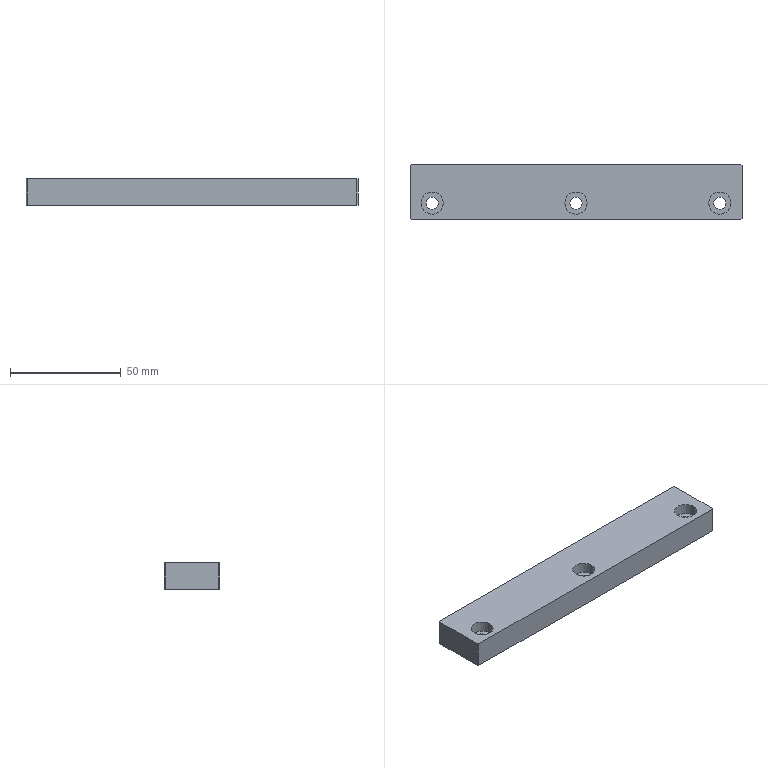Part | SolidWorks | features Chamfer 1, Extrusion 1, HoleWzd 1 | 1 solid | 25 faces | box 150 x 25 x 12 mm | volume 43317 mm3 | plane 13 | cylinder 12 | commonest cylinder face diameters 5.5 x6 10 x6
STEP:
#1=CARTESIAN_POINT('',(-5.,-5.,7.));
#2=VERTEX_POINT('',#1);
#3=CARTESIAN_POINT('',(5.,-5.,7.));
#4=VERTEX_POINT('',#3);
#5=CARTESIAN_POINT('',(0.,-5.,7.));
#6=DIRECTION('',(0.,0.,1.));
#7=DIRECTION('',(1.,0.,0.));
#8=AXIS2_PLACEMENT_3D('',#5,#6,#7);
#9=CIRCLE('',#8,5.);
#10=EDGE_CURVE('',#2,#4,#9,.T.);
#11=ORIENTED_EDGE('',*,*,#10,.F.);
#12=CARTESIAN_POINT('',(-5.,-5.,12.));
#13=VERTEX_POINT('',#12);
#14=CARTESIAN_POINT('',(-5.,-5.,12.));
#15=DIRECTION('',(0.,0.,1.));
#16=VECTOR('',#15,1000.);
#17=LINE('',#14,#16);
#18=EDGE_CURVE('',#2,#13,#17,.T.);
#19=ORIENTED_EDGE('',*,*,#18,.T.);
#20=CARTESIAN_POINT('',(5.,-5.,12.));
#21=VERTEX_POINT('',#20);
#22=CARTESIAN_POINT('',(0.,-5.,12.));
#23=DIRECTION('',(0.,0.,1.));
#24=DIRECTION('',(1.,0.,0.));
#25=AXIS2_PLACEMENT_3D('',#22,#23,#24);
#26=CIRCLE('',#25,5.);
#27=EDGE_CURVE('',#13,#21,#26,.T.);
#28=ORIENTED_EDGE('',*,*,#27,.T.);
#29=CARTESIAN_POINT('',(5.,-5.,12.));
#30=DIRECTION('',(0.,0.,1.));
#31=VECTOR('',#30,1000.);
#32=LINE('',#29,#31);
#33=EDGE_CURVE('',#4,#21,#32,.T.);
#34=ORIENTED_EDGE('',*,*,#33,.F.);
#35=EDGE_LOOP('',(#11,#19,#28,#34));
#36=FACE_OUTER_BOUND('',#35,.T.);
#37=CARTESIAN_POINT('',(0.,-5.,12.));
#38=DIRECTION('',(0.,0.,1.));
#39=DIRECTION('',(1.,0.,0.));
#40=AXIS2_PLACEMENT_3D('',#37,#38,#39);
#41=CYLINDRICAL_SURFACE('',#40,5.);
#42=ADVANCED_FACE('',(#36),#41,.F.);
#43=CARTESIAN_POINT('',(-2.75,-5.,0.));
#44=VERTEX_POINT('',#43);
#45=CARTESIAN_POINT('',(2.75,-5.,0.));
#46=VERTEX_POINT('',#45);
#47=CARTESIAN_POINT('',(0.,-5.,0.));
#48=DIRECTION('',(0.,0.,1.));
#49=DIRECTION('',(1.,0.,0.));
#50=AXIS2_PLACEMENT_3D('',#47,#48,#49);
#51=CIRCLE('',#50,2.75);
#52=EDGE_CURVE('',#44,#46,#51,.T.);
#53=ORIENTED_EDGE('',*,*,#52,.F.);
#54=CARTESIAN_POINT('',(-2.75,-5.,7.));
#55=VERTEX_POINT('',#54);
#56=CARTESIAN_POINT('',(-2.75,-5.,12.));
#57=DIRECTION('',(0.,0.,1.));
#58=VECTOR('',#57,1000.);
#59=LINE('',#56,#58);
#60=EDGE_CURVE('',#44,#55,#59,.T.);
#61=ORIENTED_EDGE('',*,*,#60,.T.);
#62=CARTESIAN_POINT('',(2.75,-5.,7.));
#63=VERTEX_POINT('',#62);
#64=CARTESIAN_POINT('',(0.,-5.,7.));
#65=DIRECTION('',(0.,0.,1.));
#66=DIRECTION('',(1.,0.,0.));
#67=AXIS2_PLACEMENT_3D('',#64,#65,#66);
#68=CIRCLE('',#67,2.75);
#69=EDGE_CURVE('',#55,#63,#68,.T.);
#70=ORIENTED_EDGE('',*,*,#69,.T.);
#71=CARTESIAN_POINT('',(2.75,-5.,12.));
#72=DIRECTION('',(0.,0.,1.));
#73=VECTOR('',#72,1000.);
#74=LINE('',#71,#73);
#75=EDGE_CURVE('',#46,#63,#74,.T.);
#76=ORIENTED_EDGE('',*,*,#75,.F.);
#77=EDGE_LOOP('',(#53,#61,#70,#76));
#78=FACE_OUTER_BOUND('',#77,.T.);
#79=CARTESIAN_POINT('',(0.,-5.,12.));
#80=DIRECTION('',(0.,0.,1.));
#81=DIRECTION('',(1.,0.,0.));
#82=AXIS2_PLACEMENT_3D('',#79,#80,#81);
#83=CYLINDRICAL_SURFACE('',#82,2.75);
#84=ADVANCED_FACE('',(#78),#83,.F.);
#85=CARTESIAN_POINT('',(-70.,-5.,7.));
#86=VERTEX_POINT('',#85);
#87=CARTESIAN_POINT('',(-60.,-5.,7.));
#88=VERTEX_POINT('',#87);
#89=CARTESIAN_POINT('',(-65.,-5.,7.));
#90=DIRECTION('',(0.,0.,1.));
#91=DIRECTION('',(1.,0.,0.));
#92=AXIS2_PLACEMENT_3D('',#89,#90,#91);
#93=CIRCLE('',#92,5.);
#94=EDGE_CURVE('',#86,#88,#93,.T.);
#95=ORIENTED_EDGE('',*,*,#94,.F.);
#96=CARTESIAN_POINT('',(-70.,-5.,12.));
#97=VERTEX_POINT('',#96);
#98=CARTESIAN_POINT('',(-70.,-5.,12.));
#99=DIRECTION('',(0.,0.,1.));
#100=VECTOR('',#99,1000.);
#101=LINE('',#98,#100);
#102=EDGE_CURVE('',#86,#97,#101,.T.);
#103=ORIENTED_EDGE('',*,*,#102,.T.);
#104=CARTESIAN_POINT('',(-60.,-5.,12.));
#105=VERTEX_POINT('',#104);
#106=CARTESIAN_POINT('',(-65.,-5.,12.));
#107=DIRECTION('',(0.,0.,1.));
#108=DIRECTION('',(1.,0.,0.));
#109=AXIS2_PLACEMENT_3D('',#106,#107,#108);
#110=CIRCLE('',#109,5.);
#111=EDGE_CURVE('',#97,#105,#110,.T.);
#112=ORIENTED_EDGE('',*,*,#111,.T.);
#113=CARTESIAN_POINT('',(-60.,-5.,12.));
#114=DIRECTION('',(0.,0.,1.));
#115=VECTOR('',#114,1000.);
#116=LINE('',#113,#115);
#117=EDGE_CURVE('',#88,#105,#116,.T.);
#118=ORIENTED_EDGE('',*,*,#117,.F.);
#119=EDGE_LOOP('',(#95,#103,#112,#118));
#120=FACE_OUTER_BOUND('',#119,.T.);
#121=CARTESIAN_POINT('',(-65.,-5.,12.));
#122=DIRECTION('',(0.,0.,1.));
#123=DIRECTION('',(1.,0.,0.));
#124=AXIS2_PLACEMENT_3D('',#121,#122,#123);
#125=CYLINDRICAL_SURFACE('',#124,5.);
#126=ADVANCED_FACE('',(#120),#125,.F.);
#127=CARTESIAN_POINT('',(-67.75,-5.,0.));
#128=VERTEX_POINT('',#127);
#129=CARTESIAN_POINT('',(-62.25,-5.,0.));
#130=VERTEX_POINT('',#129);
#131=CARTESIAN_POINT('',(-65.,-5.,0.));
#132=DIRECTION('',(0.,0.,1.));
#133=DIRECTION('',(1.,0.,0.));
#134=AXIS2_PLACEMENT_3D('',#131,#132,#133);
#135=CIRCLE('',#134,2.75);
#136=EDGE_CURVE('',#128,#130,#135,.T.);
#137=ORIENTED_EDGE('',*,*,#136,.F.);
#138=CARTESIAN_POINT('',(-67.75,-5.,7.));
#139=VERTEX_POINT('',#138);
#140=CARTESIAN_POINT('',(-67.75,-5.,12.));
#141=DIRECTION('',(0.,0.,1.));
#142=VECTOR('',#141,1000.);
#143=LINE('',#140,#142);
#144=EDGE_CURVE('',#128,#139,#143,.T.);
#145=ORIENTED_EDGE('',*,*,#144,.T.);
#146=CARTESIAN_POINT('',(-62.25,-5.,7.));
#147=VERTEX_POINT('',#146);
#148=CARTESIAN_POINT('',(-65.,-5.,7.));
#149=DIRECTION('',(0.,0.,1.));
#150=DIRECTION('',(1.,0.,0.));
#151=AXIS2_PLACEMENT_3D('',#148,#149,#150);
#152=CIRCLE('',#151,2.75);
#153=EDGE_CURVE('',#139,#147,#152,.T.);
#154=ORIENTED_EDGE('',*,*,#153,.T.);
#155=CARTESIAN_POINT('',(-62.25,-5.,12.));
#156=DIRECTION('',(0.,0.,1.));
#157=VECTOR('',#156,1000.);
#158=LINE('',#155,#157);
#159=EDGE_CURVE('',#130,#147,#158,.T.);
#160=ORIENTED_EDGE('',*,*,#159,.F.);
#161=EDGE_LOOP('',(#137,#145,#154,#160));
#162=FACE_OUTER_BOUND('',#161,.T.);
#163=CARTESIAN_POINT('',(-65.,-5.,12.));
#164=DIRECTION('',(0.,0.,1.));
#165=DIRECTION('',(1.,0.,0.));
#166=AXIS2_PLACEMENT_3D('',#163,#164,#165);
#167=CYLINDRICAL_SURFACE('',#166,2.75);
#168=ADVANCED_FACE('',(#162),#167,.F.);
#169=CARTESIAN_POINT('',(60.,-5.,7.));
#170=VERTEX_POINT('',#169);
#171=CARTESIAN_POINT('',(70.,-5.,7.));
#172=VERTEX_POINT('',#171);
#173=CARTESIAN_POINT('',(65.,-5.,7.));
#174=DIRECTION('',(0.,0.,1.));
#175=DIRECTION('',(1.,0.,0.));
#176=AXIS2_PLACEMENT_3D('',#173,#174,#175);
#177=CIRCLE('',#176,5.);
#178=EDGE_CURVE('',#170,#172,#177,.T.);
#179=ORIENTED_EDGE('',*,*,#178,.F.);
#180=CARTESIAN_POINT('',(60.,-5.,12.));
#181=VERTEX_POINT('',#180);
#182=CARTESIAN_POINT('',(60.,-5.,12.));
#183=DIRECTION('',(0.,0.,1.));
#184=VECTOR('',#183,1000.);
#185=LINE('',#182,#184);
#186=EDGE_CURVE('',#170,#181,#185,.T.);
#187=ORIENTED_EDGE('',*,*,#186,.T.);
#188=CARTESIAN_POINT('',(70.,-5.,12.));
#189=VERTEX_POINT('',#188);
#190=CARTESIAN_POINT('',(65.,-5.,12.));
#191=DIRECTION('',(0.,0.,1.));
#192=DIRECTION('',(1.,0.,0.));
#193=AXIS2_PLACEMENT_3D('',#190,#191,#192);
#194=CIRCLE('',#193,5.);
#195=EDGE_CURVE('',#181,#189,#194,.T.);
#196=ORIENTED_EDGE('',*,*,#195,.T.);
#197=CARTESIAN_POINT('',(70.,-5.,12.));
#198=DIRECTION('',(0.,0.,1.));
#199=VECTOR('',#198,1000.);
#200=LINE('',#197,#199);
#201=EDGE_CURVE('',#172,#189,#200,.T.);
#202=ORIENTED_EDGE('',*,*,#201,.F.);
#203=EDGE_LOOP('',(#179,#187,#196,#202));
#204=FACE_OUTER_BOUND('',#203,.T.);
#205=CARTESIAN_POINT('',(65.,-5.,12.));
#206=DIRECTION('',(0.,0.,1.));
#207=DIRECTION('',(1.,0.,0.));
#208=AXIS2_PLACEMENT_3D('',#205,#206,#207);
#209=CYLINDRICAL_SURFACE('',#208,5.);
#210=ADVANCED_FACE('',(#204),#209,.F.);
#211=CARTESIAN_POINT('',(62.25,-5.,0.));
#212=VERTEX_POINT('',#211);
#213=CARTESIAN_POINT('',(67.75,-5.,0.));
#214=VERTEX_POINT('',#213);
#215=CARTESIAN_POINT('',(65.,-5.,0.));
#216=DIRECTION('',(0.,0.,1.));
#217=DIRECTION('',(1.,0.,0.));
#218=AXIS2_PLACEMENT_3D('',#215,#216,#217);
#219=CIRCLE('',#218,2.75);
#220=EDGE_CURVE('',#212,#214,#219,.T.);
#221=ORIENTED_EDGE('',*,*,#220,.F.);
#222=CARTESIAN_POINT('',(62.25,-5.,7.));
#223=VERTEX_POINT('',#222);
#224=CARTESIAN_POINT('',(62.25,-5.,12.));
#225=DIRECTION('',(0.,0.,1.));
#226=VECTOR('',#225,1000.);
#227=LINE('',#224,#226);
#228=EDGE_CURVE('',#212,#223,#227,.T.);
#229=ORIENTED_EDGE('',*,*,#228,.T.);
#230=CARTESIAN_POINT('',(67.75,-5.,7.));
#231=VERTEX_POINT('',#230);
#232=CARTESIAN_POINT('',(65.,-5.,7.));
#233=DIRECTION('',(0.,0.,1.));
#234=DIRECTION('',(1.,0.,0.));
#235=AXIS2_PLACEMENT_3D('',#232,#233,#234);
#236=CIRCLE('',#235,2.75);
#237=EDGE_CURVE('',#223,#231,#236,.T.);
#238=ORIENTED_EDGE('',*,*,#237,.T.);
#239=CARTESIAN_POINT('',(67.75,-5.,12.));
#240=DIRECTION('',(0.,0.,1.));
#241=VECTOR('',#240,1000.);
#242=LINE('',#239,#241);
#243=EDGE_CURVE('',#214,#231,#242,.T.);
#244=ORIENTED_EDGE('',*,*,#243,.F.);
#245=EDGE_LOOP('',(#221,#229,#238,#244));
#246=FACE_OUTER_BOUND('',#245,.T.);
#247=CARTESIAN_POINT('',(65.,-5.,12.));
#248=DIRECTION('',(0.,0.,1.));
#249=DIRECTION('',(1.,0.,0.));
#250=AXIS2_PLACEMENT_3D('',#247,#248,#249);
#251=CYLINDRICAL_SURFACE('',#250,2.75);
#252=ADVANCED_FACE('',(#246),#251,.F.);
#253=CARTESIAN_POINT('',(75.,-12.,12.));
#254=VERTEX_POINT('',#253);
#255=CARTESIAN_POINT('',(75.,12.,12.));
#256=VERTEX_POINT('',#255);
#257=CARTESIAN_POINT('',(75.,12.5,12.));
#258=DIRECTION('',(0.,1.,0.));
#259=VECTOR('',#258,1000.);
#260=LINE('',#257,#259);
#261=EDGE_CURVE('',#254,#256,#260,.T.);
#262=ORIENTED_EDGE('',*,*,#261,.F.);
#263=CARTESIAN_POINT('',(75.,-12.,0.));
#264=VERTEX_POINT('',#263);
#265=CARTESIAN_POINT('',(75.,-12.,12.));
#266=DIRECTION('',(0.,0.,-1.));
#267=VECTOR('',#266,1000.);
#268=LINE('',#265,#267);
#269=EDGE_CURVE('',#254,#264,#268,.T.);
#270=ORIENTED_EDGE('',*,*,#269,.T.);
#271=CARTESIAN_POINT('',(75.,12.,0.));
#272=VERTEX_POINT('',#271);
#273=CARTESIAN_POINT('',(75.,12.5,0.));
#274=DIRECTION('',(0.,1.,0.));
#275=VECTOR('',#274,1000.);
#276=LINE('',#273,#275);
#277=EDGE_CURVE('',#264,#272,#276,.T.);
#278=ORIENTED_EDGE('',*,*,#277,.T.);
#279=CARTESIAN_POINT('',(75.,12.,12.));
#280=DIRECTION('',(0.,0.,1.));
#281=VECTOR('',#280,1000.);
#282=LINE('',#279,#281);
#283=EDGE_CURVE('',#272,#256,#282,.T.);
#284=ORIENTED_EDGE('',*,*,#283,.T.);
#285=EDGE_LOOP('',(#262,#270,#278,#284));
#286=FACE_OUTER_BOUND('',#285,.T.);
#287=CARTESIAN_POINT('',(75.,12.5,12.));
#288=DIRECTION('',(-1.,0.,0.));
#289=DIRECTION('',(0.,0.,1.));
#290=AXIS2_PLACEMENT_3D('',#287,#288,#289);
#291=PLANE('',#290);
#292=ADVANCED_FACE('',(#286),#291,.F.);
#293=CARTESIAN_POINT('',(74.5,12.5,12.));
#294=VERTEX_POINT('',#293);
#295=CARTESIAN_POINT('',(-74.5,12.5,12.));
#296=VERTEX_POINT('',#295);
#297=CARTESIAN_POINT('',(-75.,12.5,12.));
#298=DIRECTION('',(-1.,0.,0.));
#299=VECTOR('',#298,1000.);
#300=LINE('',#297,#299);
#301=EDGE_CURVE('',#294,#296,#300,.T.);
#302=ORIENTED_EDGE('',*,*,#301,.F.);
#303=CARTESIAN_POINT('',(74.5,12.5,0.));
#304=VERTEX_POINT('',#303);
#305=CARTESIAN_POINT('',(74.5,12.5,12.));
#306=DIRECTION('',(0.,0.,-1.));
#307=VECTOR('',#306,1000.);
#308=LINE('',#305,#307);
#309=EDGE_CURVE('',#294,#304,#308,.T.);
#310=ORIENTED_EDGE('',*,*,#309,.T.);
#311=CARTESIAN_POINT('',(-74.5,12.5,0.));
#312=VERTEX_POINT('',#311);
#313=CARTESIAN_POINT('',(-75.,12.5,0.));
#314=DIRECTION('',(-1.,0.,0.));
#315=VECTOR('',#314,1000.);
#316=LINE('',#313,#315);
#317=EDGE_CURVE('',#304,#312,#316,.T.);
#318=ORIENTED_EDGE('',*,*,#317,.T.);
#319=CARTESIAN_POINT('',(-74.5,12.5,12.));
#320=DIRECTION('',(0.,0.,1.));
#321=VECTOR('',#320,1000.);
#322=LINE('',#319,#321);
#323=EDGE_CURVE('',#312,#296,#322,.T.);
#324=ORIENTED_EDGE('',*,*,#323,.T.);
#325=EDGE_LOOP('',(#302,#310,#318,#324));
#326=FACE_OUTER_BOUND('',#325,.T.);
#327=CARTESIAN_POINT('',(-75.,12.5,12.));
#328=DIRECTION('',(0.,-1.,0.));
#329=DIRECTION('',(0.,0.,-1.));
#330=AXIS2_PLACEMENT_3D('',#327,#328,#329);
#331=PLANE('',#330);
#332=ADVANCED_FACE('',(#326),#331,.F.);
#333=CARTESIAN_POINT('',(-75.,12.,12.));
#334=VERTEX_POINT('',#333);
#335=CARTESIAN_POINT('',(-75.,-12.,12.));
#336=VERTEX_POINT('',#335);
#337=CARTESIAN_POINT('',(-75.,12.5,12.));
#338=DIRECTION('',(0.,-1.,0.));
#339=VECTOR('',#338,1000.);
#340=LINE('',#337,#339);
#341=EDGE_CURVE('',#334,#336,#340,.T.);
#342=ORIENTED_EDGE('',*,*,#341,.F.);
#343=CARTESIAN_POINT('',(-75.,12.,0.));
#344=VERTEX_POINT('',#343);
#345=CARTESIAN_POINT('',(-75.,12.,12.));
#346=DIRECTION('',(0.,0.,-1.));
#347=VECTOR('',#346,1000.);
#348=LINE('',#345,#347);
#349=EDGE_CURVE('',#334,#344,#348,.T.);
#350=ORIENTED_EDGE('',*,*,#349,.T.);
#351=CARTESIAN_POINT('',(-75.,-12.,0.));
#352=VERTEX_POINT('',#351);
#353=CARTESIAN_POINT('',(-75.,12.5,0.));
#354=DIRECTION('',(0.,-1.,0.));
#355=VECTOR('',#354,1000.);
#356=LINE('',#353,#355);
#357=EDGE_CURVE('',#344,#352,#356,.T.);
#358=ORIENTED_EDGE('',*,*,#357,.T.);
#359=CARTESIAN_POINT('',(-75.,-12.,12.));
#360=DIRECTION('',(0.,0.,1.));
#361=VECTOR('',#360,1000.);
#362=LINE('',#359,#361);
#363=EDGE_CURVE('',#352,#336,#362,.T.);
#364=ORIENTED_EDGE('',*,*,#363,.T.);
#365=EDGE_LOOP('',(#342,#350,#358,#364));
#366=FACE_OUTER_BOUND('',#365,.T.);
#367=CARTESIAN_POINT('',(-75.,12.5,12.));
#368=DIRECTION('',(1.,0.,0.));
#369=DIRECTION('',(0.,0.,-1.));
#370=AXIS2_PLACEMENT_3D('',#367,#368,#369);
#371=PLANE('',#370);
#372=ADVANCED_FACE('',(#366),#371,.F.);
#373=CARTESIAN_POINT('',(-74.5,-12.5,0.));
#374=VERTEX_POINT('',#373);
#375=CARTESIAN_POINT('',(74.5,-12.5,0.));
#376=VERTEX_POINT('',#375);
#377=CARTESIAN_POINT('',(-75.,-12.5,0.));
#378=DIRECTION('',(1.,0.,0.));
#379=VECTOR('',#378,1000.);
#380=LINE('',#377,#379);
#381=EDGE_CURVE('',#374,#376,#380,.T.);
#382=ORIENTED_EDGE('',*,*,#381,.T.);
#383=CARTESIAN_POINT('',(74.5,-12.5,12.));
#384=VERTEX_POINT('',#383);
#385=CARTESIAN_POINT('',(74.5,-12.5,12.));
#386=DIRECTION('',(0.,0.,1.));
#387=VECTOR('',#386,1000.);
#388=LINE('',#385,#387);
#389=EDGE_CURVE('',#376,#384,#388,.T.);
#390=ORIENTED_EDGE('',*,*,#389,.T.);
#391=CARTESIAN_POINT('',(-74.5,-12.5,12.));
#392=VERTEX_POINT('',#391);
#393=CARTESIAN_POINT('',(-75.,-12.5,12.));
#394=DIRECTION('',(1.,0.,0.));
#395=VECTOR('',#394,1000.);
#396=LINE('',#393,#395);
#397=EDGE_CURVE('',#392,#384,#396,.T.);
#398=ORIENTED_EDGE('',*,*,#397,.F.);
#399=CARTESIAN_POINT('',(-74.5,-12.5,12.));
#400=DIRECTION('',(0.,0.,-1.));
#401=VECTOR('',#400,1000.);
#402=LINE('',#399,#401);
#403=EDGE_CURVE('',#392,#374,#402,.T.);
#404=ORIENTED_EDGE('',*,*,#403,.T.);
#405=EDGE_LOOP('',(#382,#390,#398,#404));
#406=FACE_OUTER_BOUND('',#405,.T.);
#407=CARTESIAN_POINT('',(-75.,-12.5,12.));
#408=DIRECTION('',(0.,1.,0.));
#409=DIRECTION('',(0.,0.,1.));
#410=AXIS2_PLACEMENT_3D('',#407,#408,#409);
#411=PLANE('',#410);
#412=ADVANCED_FACE('',(#406),#411,.F.);
#413=CARTESIAN_POINT('',(0.,-5.,12.));
#414=DIRECTION('',(0.,0.,1.));
#415=DIRECTION('',(1.,0.,0.));
#416=AXIS2_PLACEMENT_3D('',#413,#414,#415);
#417=CIRCLE('',#416,5.);
#418=EDGE_CURVE('',#21,#13,#417,.T.);
#419=ORIENTED_EDGE('',*,*,#418,.F.);
#420=ORIENTED_EDGE('',*,*,#27,.F.);
#421=EDGE_LOOP('',(#419,#420));
#422=FACE_BOUND('',#421,.T.);
#423=CARTESIAN_POINT('',(-65.,-5.,12.));
#424=DIRECTION('',(0.,0.,1.));
#425=DIRECTION('',(1.,0.,0.));
#426=AXIS2_PLACEMENT_3D('',#423,#424,#425);
#427=CIRCLE('',#426,5.);
#428=EDGE_CURVE('',#105,#97,#427,.T.);
#429=ORIENTED_EDGE('',*,*,#428,.F.);
#430=ORIENTED_EDGE('',*,*,#111,.F.);
#431=EDGE_LOOP('',(#429,#430));
#432=FACE_BOUND('',#431,.T.);
#433=CARTESIAN_POINT('',(65.,-5.,12.));
#434=DIRECTION('',(0.,0.,1.));
#435=DIRECTION('',(1.,0.,0.));
#436=AXIS2_PLACEMENT_3D('',#433,#434,#435);
#437=CIRCLE('',#436,5.);
#438=EDGE_CURVE('',#189,#181,#437,.T.);
#439=ORIENTED_EDGE('',*,*,#438,.F.);
#440=ORIENTED_EDGE('',*,*,#195,.F.);
#441=EDGE_LOOP('',(#439,#440));
#442=FACE_BOUND('',#441,.T.);
#443=ORIENTED_EDGE('',*,*,#397,.T.);
#444=CARTESIAN_POINT('',(74.75,-12.25,12.));
#445=DIRECTION('',(0.7071,0.7071,0.));
#446=VECTOR('',#445,1000.);
#447=LINE('',#444,#446);
#448=EDGE_CURVE('',#384,#254,#447,.T.);
#449=ORIENTED_EDGE('',*,*,#448,.T.);
#450=ORIENTED_EDGE('',*,*,#261,.T.);
#451=CARTESIAN_POINT('',(87.25,-0.25,12.));
#452=DIRECTION('',(-0.7071,0.7071,0.));
#453=VECTOR('',#452,1000.);
#454=LINE('',#451,#453);
#455=EDGE_CURVE('',#256,#294,#454,.T.);
#456=ORIENTED_EDGE('',*,*,#455,.T.);
#457=ORIENTED_EDGE('',*,*,#301,.T.);
#458=CARTESIAN_POINT('',(-12.25,74.75,12.));
#459=DIRECTION('',(-0.7071,-0.7071,0.));
#460=VECTOR('',#459,1000.);
#461=LINE('',#458,#460);
#462=EDGE_CURVE('',#296,#334,#461,.T.);
#463=ORIENTED_EDGE('',*,*,#462,.T.);
#464=ORIENTED_EDGE('',*,*,#341,.T.);
#465=CARTESIAN_POINT('',(0.25,-87.25,12.));
#466=DIRECTION('',(0.7071,-0.7071,0.));
#467=VECTOR('',#466,1000.);
#468=LINE('',#465,#467);
#469=EDGE_CURVE('',#336,#392,#468,.T.);
#470=ORIENTED_EDGE('',*,*,#469,.T.);
#471=EDGE_LOOP('',(#443,#449,#450,#456,#457,#463,#464,#470));
#472=FACE_OUTER_BOUND('',#471,.T.);
#473=CARTESIAN_POINT('',(75.,-12.5,12.));
#474=DIRECTION('',(0.,0.,1.));
#475=DIRECTION('',(1.,0.,0.));
#476=AXIS2_PLACEMENT_3D('',#473,#474,#475);
#477=PLANE('',#476);
#478=ADVANCED_FACE('',(#422,#432,#442,#472),#477,.T.);
#479=CARTESIAN_POINT('',(0.,-5.,0.));
#480=DIRECTION('',(0.,0.,1.));
#481=DIRECTION('',(1.,0.,0.));
#482=AXIS2_PLACEMENT_3D('',#479,#480,#481);
#483=CIRCLE('',#482,2.75);
#484=EDGE_CURVE('',#46,#44,#483,.T.);
#485=ORIENTED_EDGE('',*,*,#484,.T.);
#486=ORIENTED_EDGE('',*,*,#52,.T.);
#487=EDGE_LOOP('',(#485,#486));
#488=FACE_BOUND('',#487,.T.);
#489=CARTESIAN_POINT('',(-65.,-5.,0.));
#490=DIRECTION('',(0.,0.,1.));
#491=DIRECTION('',(1.,0.,0.));
#492=AXIS2_PLACEMENT_3D('',#489,#490,#491);
#493=CIRCLE('',#492,2.75);
#494=EDGE_CURVE('',#130,#128,#493,.T.);
#495=ORIENTED_EDGE('',*,*,#494,.T.);
#496=ORIENTED_EDGE('',*,*,#136,.T.);
#497=EDGE_LOOP('',(#495,#496));
#498=FACE_BOUND('',#497,.T.);
#499=CARTESIAN_POINT('',(65.,-5.,0.));
#500=DIRECTION('',(0.,0.,1.));
#501=DIRECTION('',(1.,0.,0.));
#502=AXIS2_PLACEMENT_3D('',#499,#500,#501);
#503=CIRCLE('',#502,2.75);
#504=EDGE_CURVE('',#214,#212,#503,.T.);
#505=ORIENTED_EDGE('',*,*,#504,.T.);
#506=ORIENTED_EDGE('',*,*,#220,.T.);
#507=EDGE_LOOP('',(#505,#506));
#508=FACE_BOUND('',#507,.T.);
#509=ORIENTED_EDGE('',*,*,#277,.F.);
#510=CARTESIAN_POINT('',(75.,-12.,0.));
#511=DIRECTION('',(-0.7071,-0.7071,0.));
#512=VECTOR('',#511,1000.);
#513=LINE('',#510,#512);
#514=EDGE_CURVE('',#264,#376,#513,.T.);
#515=ORIENTED_EDGE('',*,*,#514,.T.);
#516=ORIENTED_EDGE('',*,*,#381,.F.);
#517=CARTESIAN_POINT('',(-74.5,-12.5,0.));
#518=DIRECTION('',(-0.7071,0.7071,0.));
#519=VECTOR('',#518,1000.);
#520=LINE('',#517,#519);
#521=EDGE_CURVE('',#374,#352,#520,.T.);
#522=ORIENTED_EDGE('',*,*,#521,.T.);
#523=ORIENTED_EDGE('',*,*,#357,.F.);
#524=CARTESIAN_POINT('',(-75.,12.,0.));
#525=DIRECTION('',(0.7071,0.7071,0.));
#526=VECTOR('',#525,1000.);
#527=LINE('',#524,#526);
#528=EDGE_CURVE('',#344,#312,#527,.T.);
#529=ORIENTED_EDGE('',*,*,#528,.T.);
#530=ORIENTED_EDGE('',*,*,#317,.F.);
#531=CARTESIAN_POINT('',(74.5,12.5,0.));
#532=DIRECTION('',(0.7071,-0.7071,0.));
#533=VECTOR('',#532,1000.);
#534=LINE('',#531,#533);
#535=EDGE_CURVE('',#304,#272,#534,.T.);
#536=ORIENTED_EDGE('',*,*,#535,.T.);
#537=EDGE_LOOP('',(#509,#515,#516,#522,#523,#529,#530,#536));
#538=FACE_OUTER_BOUND('',#537,.T.);
#539=CARTESIAN_POINT('',(75.,-12.5,0.));
#540=DIRECTION('',(0.,0.,1.));
#541=DIRECTION('',(1.,0.,0.));
#542=AXIS2_PLACEMENT_3D('',#539,#540,#541);
#543=PLANE('',#542);
#544=ADVANCED_FACE('',(#488,#498,#508,#538),#543,.F.);
#545=ORIENTED_EDGE('',*,*,#228,.F.);
#546=ORIENTED_EDGE('',*,*,#504,.F.);
#547=ORIENTED_EDGE('',*,*,#243,.T.);
#548=CARTESIAN_POINT('',(65.,-5.,7.));
#549=DIRECTION('',(0.,0.,1.));
#550=DIRECTION('',(1.,0.,0.));
#551=AXIS2_PLACEMENT_3D('',#548,#549,#550);
#552=CIRCLE('',#551,2.75);
#553=EDGE_CURVE('',#231,#223,#552,.T.);
#554=ORIENTED_EDGE('',*,*,#553,.T.);
#555=EDGE_LOOP('',(#545,#546,#547,#554));
#556=FACE_OUTER_BOUND('',#555,.T.);
#557=CARTESIAN_POINT('',(65.,-5.,12.));
#558=DIRECTION('',(0.,0.,1.));
#559=DIRECTION('',(1.,0.,0.));
#560=AXIS2_PLACEMENT_3D('',#557,#558,#559);
#561=CYLINDRICAL_SURFACE('',#560,2.75);
#562=ADVANCED_FACE('',(#556),#561,.F.);
#563=ORIENTED_EDGE('',*,*,#553,.F.);
#564=ORIENTED_EDGE('',*,*,#237,.F.);
#565=EDGE_LOOP('',(#563,#564));
#566=FACE_BOUND('',#565,.T.);
#567=CARTESIAN_POINT('',(65.,-5.,7.));
#568=DIRECTION('',(0.,0.,1.));
#569=DIRECTION('',(1.,0.,0.));
#570=AXIS2_PLACEMENT_3D('',#567,#568,#569);
#571=CIRCLE('',#570,5.);
#572=EDGE_CURVE('',#172,#170,#571,.T.);
#573=ORIENTED_EDGE('',*,*,#572,.T.);
#574=ORIENTED_EDGE('',*,*,#178,.T.);
#575=EDGE_LOOP('',(#573,#574));
#576=FACE_OUTER_BOUND('',#575,.T.);
#577=CARTESIAN_POINT('',(67.75,-5.,7.));
#578=DIRECTION('',(0.,0.,-1.));
#579=DIRECTION('',(-1.,0.,0.));
#580=AXIS2_PLACEMENT_3D('',#577,#578,#579);
#581=PLANE('',#580);
#582=ADVANCED_FACE('',(#566,#576),#581,.F.);
#583=ORIENTED_EDGE('',*,*,#186,.F.);
#584=ORIENTED_EDGE('',*,*,#572,.F.);
#585=ORIENTED_EDGE('',*,*,#201,.T.);
#586=ORIENTED_EDGE('',*,*,#438,.T.);
#587=EDGE_LOOP('',(#583,#584,#585,#586));
#588=FACE_OUTER_BOUND('',#587,.T.);
#589=CARTESIAN_POINT('',(65.,-5.,12.));
#590=DIRECTION('',(0.,0.,1.));
#591=DIRECTION('',(1.,0.,0.));
#592=AXIS2_PLACEMENT_3D('',#589,#590,#591);
#593=CYLINDRICAL_SURFACE('',#592,5.);
#594=ADVANCED_FACE('',(#588),#593,.F.);
#595=ORIENTED_EDGE('',*,*,#144,.F.);
#596=ORIENTED_EDGE('',*,*,#494,.F.);
#597=ORIENTED_EDGE('',*,*,#159,.T.);
#598=CARTESIAN_POINT('',(-65.,-5.,7.));
#599=DIRECTION('',(0.,0.,1.));
#600=DIRECTION('',(1.,0.,0.));
#601=AXIS2_PLACEMENT_3D('',#598,#599,#600);
#602=CIRCLE('',#601,2.75);
#603=EDGE_CURVE('',#147,#139,#602,.T.);
#604=ORIENTED_EDGE('',*,*,#603,.T.);
#605=EDGE_LOOP('',(#595,#596,#597,#604));
#606=FACE_OUTER_BOUND('',#605,.T.);
#607=CARTESIAN_POINT('',(-65.,-5.,12.));
#608=DIRECTION('',(0.,0.,1.));
#609=DIRECTION('',(1.,0.,0.));
#610=AXIS2_PLACEMENT_3D('',#607,#608,#609);
#611=CYLINDRICAL_SURFACE('',#610,2.75);
#612=ADVANCED_FACE('',(#606),#611,.F.);
#613=ORIENTED_EDGE('',*,*,#603,.F.);
#614=ORIENTED_EDGE('',*,*,#153,.F.);
#615=EDGE_LOOP('',(#613,#614));
#616=FACE_BOUND('',#615,.T.);
#617=CARTESIAN_POINT('',(-65.,-5.,7.));
#618=DIRECTION('',(0.,0.,1.));
#619=DIRECTION('',(1.,0.,0.));
#620=AXIS2_PLACEMENT_3D('',#617,#618,#619);
#621=CIRCLE('',#620,5.);
#622=EDGE_CURVE('',#88,#86,#621,.T.);
#623=ORIENTED_EDGE('',*,*,#622,.T.);
#624=ORIENTED_EDGE('',*,*,#94,.T.);
#625=EDGE_LOOP('',(#623,#624));
#626=FACE_OUTER_BOUND('',#625,.T.);
#627=CARTESIAN_POINT('',(-62.25,-5.,7.));
#628=DIRECTION('',(0.,0.,-1.));
#629=DIRECTION('',(-1.,0.,0.));
#630=AXIS2_PLACEMENT_3D('',#627,#628,#629);
#631=PLANE('',#630);
#632=ADVANCED_FACE('',(#616,#626),#631,.F.);
#633=ORIENTED_EDGE('',*,*,#102,.F.);
#634=ORIENTED_EDGE('',*,*,#622,.F.);
#635=ORIENTED_EDGE('',*,*,#117,.T.);
#636=ORIENTED_EDGE('',*,*,#428,.T.);
#637=EDGE_LOOP('',(#633,#634,#635,#636));
#638=FACE_OUTER_BOUND('',#637,.T.);
#639=CARTESIAN_POINT('',(-65.,-5.,12.));
#640=DIRECTION('',(0.,0.,1.));
#641=DIRECTION('',(1.,0.,0.));
#642=AXIS2_PLACEMENT_3D('',#639,#640,#641);
#643=CYLINDRICAL_SURFACE('',#642,5.);
#644=ADVANCED_FACE('',(#638),#643,.F.);
#645=ORIENTED_EDGE('',*,*,#60,.F.);
#646=ORIENTED_EDGE('',*,*,#484,.F.);
#647=ORIENTED_EDGE('',*,*,#75,.T.);
#648=CARTESIAN_POINT('',(0.,-5.,7.));
#649=DIRECTION('',(0.,0.,1.));
#650=DIRECTION('',(1.,0.,0.));
#651=AXIS2_PLACEMENT_3D('',#648,#649,#650);
#652=CIRCLE('',#651,2.75);
#653=EDGE_CURVE('',#63,#55,#652,.T.);
#654=ORIENTED_EDGE('',*,*,#653,.T.);
#655=EDGE_LOOP('',(#645,#646,#647,#654));
#656=FACE_OUTER_BOUND('',#655,.T.);
#657=CARTESIAN_POINT('',(0.,-5.,12.));
#658=DIRECTION('',(0.,0.,1.));
#659=DIRECTION('',(1.,0.,0.));
#660=AXIS2_PLACEMENT_3D('',#657,#658,#659);
#661=CYLINDRICAL_SURFACE('',#660,2.75);
#662=ADVANCED_FACE('',(#656),#661,.F.);
#663=ORIENTED_EDGE('',*,*,#653,.F.);
#664=ORIENTED_EDGE('',*,*,#69,.F.);
#665=EDGE_LOOP('',(#663,#664));
#666=FACE_BOUND('',#665,.T.);
#667=CARTESIAN_POINT('',(0.,-5.,7.));
#668=DIRECTION('',(0.,0.,1.));
#669=DIRECTION('',(1.,0.,0.));
#670=AXIS2_PLACEMENT_3D('',#667,#668,#669);
#671=CIRCLE('',#670,5.);
#672=EDGE_CURVE('',#4,#2,#671,.T.);
#673=ORIENTED_EDGE('',*,*,#672,.T.);
#674=ORIENTED_EDGE('',*,*,#10,.T.);
#675=EDGE_LOOP('',(#673,#674));
#676=FACE_OUTER_BOUND('',#675,.T.);
#677=CARTESIAN_POINT('',(2.75,-5.,7.));
#678=DIRECTION('',(0.,0.,-1.));
#679=DIRECTION('',(-1.,0.,0.));
#680=AXIS2_PLACEMENT_3D('',#677,#678,#679);
#681=PLANE('',#680);
#682=ADVANCED_FACE('',(#666,#676),#681,.F.);
#683=ORIENTED_EDGE('',*,*,#18,.F.);
#684=ORIENTED_EDGE('',*,*,#672,.F.);
#685=ORIENTED_EDGE('',*,*,#33,.T.);
#686=ORIENTED_EDGE('',*,*,#418,.T.);
#687=EDGE_LOOP('',(#683,#684,#685,#686));
#688=FACE_OUTER_BOUND('',#687,.T.);
#689=CARTESIAN_POINT('',(0.,-5.,12.));
#690=DIRECTION('',(0.,0.,1.));
#691=DIRECTION('',(1.,0.,0.));
#692=AXIS2_PLACEMENT_3D('',#689,#690,#691);
#693=CYLINDRICAL_SURFACE('',#692,5.);
#694=ADVANCED_FACE('',(#688),#693,.F.);
#695=ORIENTED_EDGE('',*,*,#448,.F.);
#696=ORIENTED_EDGE('',*,*,#389,.F.);
#697=ORIENTED_EDGE('',*,*,#514,.F.);
#698=ORIENTED_EDGE('',*,*,#269,.F.);
#699=EDGE_LOOP('',(#695,#696,#697,#698));
#700=FACE_OUTER_BOUND('',#699,.T.);
#701=CARTESIAN_POINT('',(75.,-12.,12.));
#702=DIRECTION('',(-0.7071,0.7071,0.));
#703=DIRECTION('',(-0.7071,-0.7071,0.));
#704=AXIS2_PLACEMENT_3D('',#701,#702,#703);
#705=PLANE('',#704);
#706=ADVANCED_FACE('',(#700),#705,.F.);
#707=ORIENTED_EDGE('',*,*,#455,.F.);
#708=ORIENTED_EDGE('',*,*,#283,.F.);
#709=ORIENTED_EDGE('',*,*,#535,.F.);
#710=ORIENTED_EDGE('',*,*,#309,.F.);
#711=EDGE_LOOP('',(#707,#708,#709,#710));
#712=FACE_OUTER_BOUND('',#711,.T.);
#713=CARTESIAN_POINT('',(74.5,12.5,12.));
#714=DIRECTION('',(-0.7071,-0.7071,0.));
#715=DIRECTION('',(0.7071,-0.7071,0.));
#716=AXIS2_PLACEMENT_3D('',#713,#714,#715);
#717=PLANE('',#716);
#718=ADVANCED_FACE('',(#712),#717,.F.);
#719=ORIENTED_EDGE('',*,*,#462,.F.);
#720=ORIENTED_EDGE('',*,*,#323,.F.);
#721=ORIENTED_EDGE('',*,*,#528,.F.);
#722=ORIENTED_EDGE('',*,*,#349,.F.);
#723=EDGE_LOOP('',(#719,#720,#721,#722));
#724=FACE_OUTER_BOUND('',#723,.T.);
#725=CARTESIAN_POINT('',(-75.,12.,12.));
#726=DIRECTION('',(0.7071,-0.7071,0.));
#727=DIRECTION('',(0.7071,0.7071,0.));
#728=AXIS2_PLACEMENT_3D('',#725,#726,#727);
#729=PLANE('',#728);
#730=ADVANCED_FACE('',(#724),#729,.F.);
#731=ORIENTED_EDGE('',*,*,#469,.F.);
#732=ORIENTED_EDGE('',*,*,#363,.F.);
#733=ORIENTED_EDGE('',*,*,#521,.F.);
#734=ORIENTED_EDGE('',*,*,#403,.F.);
#735=EDGE_LOOP('',(#731,#732,#733,#734));
#736=FACE_OUTER_BOUND('',#735,.T.);
#737=CARTESIAN_POINT('',(-74.5,-12.5,12.));
#738=DIRECTION('',(0.7071,0.7071,0.));
#739=DIRECTION('',(-0.7071,0.7071,0.));
#740=AXIS2_PLACEMENT_3D('',#737,#738,#739);
#741=PLANE('',#740);
#742=ADVANCED_FACE('',(#736),#741,.F.);
#743=CLOSED_SHELL('',(#42,#84,#126,#168,#210,#252,#292,#332,#372,#412,#478,#544,#562,#582,#594,#612,#632,#644,#662,#682,#694,#706,#718,#730,#742));
#744=MANIFOLD_SOLID_BREP('',#743);
#745=CARTESIAN_POINT('',(0.,0.,0.));
#746=DIRECTION('',(0.,0.,1.));
#747=DIRECTION('',(1.,0.,0.));
#748=AXIS2_PLACEMENT_3D('',#745,#746,#747);
#749=(LENGTH_UNIT()NAMED_UNIT(*)SI_UNIT(.MILLI.,.METRE.));
#750=UNCERTAINTY_MEASURE_WITH_UNIT(LENGTH_MEASURE(0.00001),#749,'','');
#751=(NAMED_UNIT(*)PLANE_ANGLE_UNIT()SI_UNIT($,.RADIAN.));
#752=(NAMED_UNIT(*)SI_UNIT($,.STERADIAN.)SOLID_ANGLE_UNIT());
#753=(GEOMETRIC_REPRESENTATION_CONTEXT(3)GLOBAL_UNCERTAINTY_ASSIGNED_CONTEXT((#750))GLOBAL_UNIT_ASSIGNED_CONTEXT((#749,#751,#752))REPRESENTATION_CONTEXT('',''));
#754=ADVANCED_BREP_SHAPE_REPRESENTATION('',(#744,#748),#753);